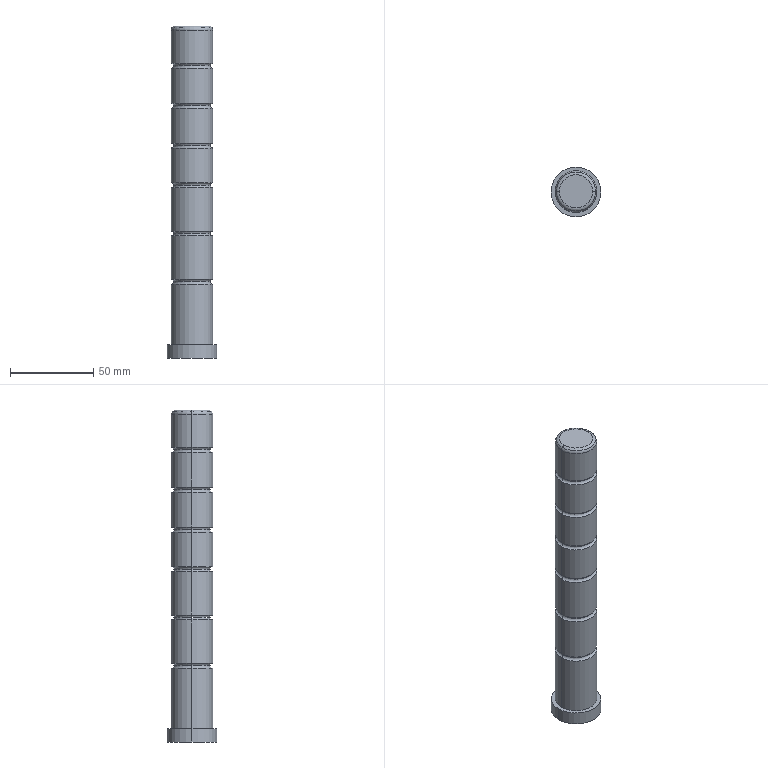Part | Creo | 1 solid | 54 faces | box 30 x 30 x 200 mm | volume 94808 mm3 | torus 28 | cylinder 20 | plane 4 | cone 2 | commonest cylinder face diameters 25 x14 10.2 x2 12 x2 30 x2
STEP:
#1=CARTESIAN_POINT('',(147.5,-266.,-182.));
#2=VERTEX_POINT('',#1);
#3=CARTESIAN_POINT('',(172.5,-266.,-182.));
#4=VERTEX_POINT('',#3);
#5=CARTESIAN_POINT('',(160.,-266.,-182.));
#6=DIRECTION('',(0.,0.,-1.));
#7=DIRECTION('',(-1.,0.,0.));
#8=AXIS2_PLACEMENT_3D('',#5,#6,#7);
#9=CIRCLE('',#8,12.5);
#10=EDGE_CURVE('',#2,#4,#9,.T.);
#11=ORIENTED_EDGE('',*,*,#10,.T.);
#12=CARTESIAN_POINT('',(172.5,-266.,-161.));
#13=VERTEX_POINT('',#12);
#14=CARTESIAN_POINT('',(172.5,-266.,-161.));
#15=DIRECTION('',(0.,0.,-1.));
#16=VECTOR('',#15,21.);
#17=LINE('',#14,#16);
#18=EDGE_CURVE('',#13,#4,#17,.T.);
#19=ORIENTED_EDGE('',*,*,#18,.F.);
#20=CARTESIAN_POINT('',(147.5,-266.,-161.));
#21=VERTEX_POINT('',#20);
#22=CARTESIAN_POINT('',(160.,-266.,-161.));
#23=DIRECTION('',(0.,0.,1.));
#24=DIRECTION('',(1.,0.,0.));
#25=AXIS2_PLACEMENT_3D('',#22,#23,#24);
#26=CIRCLE('',#25,12.5);
#27=EDGE_CURVE('',#13,#21,#26,.T.);
#28=ORIENTED_EDGE('',*,*,#27,.T.);
#29=CARTESIAN_POINT('',(147.5,-266.,-161.));
#30=DIRECTION('',(0.,0.,-1.));
#31=VECTOR('',#30,21.);
#32=LINE('',#29,#31);
#33=EDGE_CURVE('',#21,#2,#32,.T.);
#34=ORIENTED_EDGE('',*,*,#33,.T.);
#35=EDGE_LOOP('',(#11,#19,#28,#34));
#36=FACE_OUTER_BOUND('',#35,.F.);
#37=CARTESIAN_POINT('',(160.,-266.,-135.5));
#38=DIRECTION('',(0.,0.,-1.));
#39=DIRECTION('',(-1.,0.,0.));
#40=AXIS2_PLACEMENT_3D('',#37,#38,#39);
#41=CYLINDRICAL_SURFACE('',#40,12.5);
#42=ADVANCED_FACE('',(#36),#41,.T.);
#43=ORIENTED_EDGE('',*,*,#10,.F.);
#44=CARTESIAN_POINT('',(149.,-266.,-183.5));
#45=VERTEX_POINT('',#44);
#46=CARTESIAN_POINT('',(147.5,-266.,-183.5));
#47=DIRECTION('',(0.,1.,0.));
#48=DIRECTION('',(0.,0.,1.));
#49=AXIS2_PLACEMENT_3D('',#46,#47,#48);
#50=CIRCLE('',#49,1.5);
#51=EDGE_CURVE('',#2,#45,#50,.T.);
#52=ORIENTED_EDGE('',*,*,#51,.T.);
#53=CARTESIAN_POINT('',(171.,-266.,-183.5));
#54=VERTEX_POINT('',#53);
#55=CARTESIAN_POINT('',(160.,-266.,-183.5));
#56=DIRECTION('',(0.,0.,1.));
#57=DIRECTION('',(1.,0.,0.));
#58=AXIS2_PLACEMENT_3D('',#55,#56,#57);
#59=CIRCLE('',#58,11.);
#60=EDGE_CURVE('',#54,#45,#59,.T.);
#61=ORIENTED_EDGE('',*,*,#60,.F.);
#62=CARTESIAN_POINT('',(172.5,-266.,-183.5));
#63=DIRECTION('',(0.,-1.,0.));
#64=DIRECTION('',(0.,0.,1.));
#65=AXIS2_PLACEMENT_3D('',#62,#63,#64);
#66=CIRCLE('',#65,1.5);
#67=EDGE_CURVE('',#4,#54,#66,.T.);
#68=ORIENTED_EDGE('',*,*,#67,.F.);
#69=EDGE_LOOP('',(#43,#52,#61,#68));
#70=FACE_OUTER_BOUND('',#69,.F.);
#71=CARTESIAN_POINT('',(160.,-266.,-183.5));
#72=DIRECTION('',(0.,0.,1.));
#73=DIRECTION('',(1.,0.,0.));
#74=AXIS2_PLACEMENT_3D('',#71,#72,#73);
#75=TOROIDAL_SURFACE('',#74,12.5,1.5);
#76=ADVANCED_FACE('',(#70),#75,.F.);
#77=CARTESIAN_POINT('',(160.,-266.,-182.));
#78=DIRECTION('',(0.,0.,-1.));
#79=DIRECTION('',(1.,0.,0.));
#80=AXIS2_PLACEMENT_3D('',#77,#78,#79);
#81=CIRCLE('',#80,12.5);
#82=EDGE_CURVE('',#4,#2,#81,.T.);
#83=ORIENTED_EDGE('',*,*,#82,.F.);
#84=ORIENTED_EDGE('',*,*,#67,.T.);
#85=CARTESIAN_POINT('',(160.,-266.,-183.5));
#86=DIRECTION('',(0.,0.,1.));
#87=DIRECTION('',(-1.,0.,0.));
#88=AXIS2_PLACEMENT_3D('',#85,#86,#87);
#89=CIRCLE('',#88,11.);
#90=EDGE_CURVE('',#45,#54,#89,.T.);
#91=ORIENTED_EDGE('',*,*,#90,.F.);
#92=ORIENTED_EDGE('',*,*,#51,.F.);
#93=EDGE_LOOP('',(#83,#84,#91,#92));
#94=FACE_OUTER_BOUND('',#93,.F.);
#95=CARTESIAN_POINT('',(160.,-266.,-183.5));
#96=DIRECTION('',(0.,0.,1.));
#97=DIRECTION('',(1.,0.,0.));
#98=AXIS2_PLACEMENT_3D('',#95,#96,#97);
#99=TOROIDAL_SURFACE('',#98,12.5,1.5);
#100=ADVANCED_FACE('',(#94),#99,.F.);
#101=ORIENTED_EDGE('',*,*,#82,.T.);
#102=ORIENTED_EDGE('',*,*,#33,.F.);
#103=CARTESIAN_POINT('',(160.,-266.,-161.));
#104=DIRECTION('',(0.,0.,1.));
#105=DIRECTION('',(-1.,0.,0.));
#106=AXIS2_PLACEMENT_3D('',#103,#104,#105);
#107=CIRCLE('',#106,12.5);
#108=EDGE_CURVE('',#21,#13,#107,.T.);
#109=ORIENTED_EDGE('',*,*,#108,.T.);
#110=ORIENTED_EDGE('',*,*,#18,.T.);
#111=EDGE_LOOP('',(#101,#102,#109,#110));
#112=FACE_OUTER_BOUND('',#111,.F.);
#113=CARTESIAN_POINT('',(160.,-266.,-135.5));
#114=DIRECTION('',(0.,0.,-1.));
#115=DIRECTION('',(-1.,0.,0.));
#116=AXIS2_PLACEMENT_3D('',#113,#114,#115);
#117=CYLINDRICAL_SURFACE('',#116,12.5);
#118=ADVANCED_FACE('',(#112),#117,.T.);
#119=ORIENTED_EDGE('',*,*,#108,.F.);
#120=CARTESIAN_POINT('',(149.,-266.,-159.5));
#121=VERTEX_POINT('',#120);
#122=CARTESIAN_POINT('',(147.5,-266.,-159.5));
#123=DIRECTION('',(0.,1.,0.));
#124=DIRECTION('',(1.,0.,0.));
#125=AXIS2_PLACEMENT_3D('',#122,#123,#124);
#126=CIRCLE('',#125,1.5);
#127=EDGE_CURVE('',#121,#21,#126,.T.);
#128=ORIENTED_EDGE('',*,*,#127,.F.);
#129=CARTESIAN_POINT('',(171.,-266.,-159.5));
#130=VERTEX_POINT('',#129);
#131=CARTESIAN_POINT('',(160.,-266.,-159.5));
#132=DIRECTION('',(0.,0.,1.));
#133=DIRECTION('',(-1.,0.,0.));
#134=AXIS2_PLACEMENT_3D('',#131,#132,#133);
#135=CIRCLE('',#134,11.);
#136=EDGE_CURVE('',#121,#130,#135,.T.);
#137=ORIENTED_EDGE('',*,*,#136,.T.);
#138=CARTESIAN_POINT('',(172.5,-266.,-159.5));
#139=DIRECTION('',(0.,-1.,0.));
#140=DIRECTION('',(-1.,0.,0.));
#141=AXIS2_PLACEMENT_3D('',#138,#139,#140);
#142=CIRCLE('',#141,1.5);
#143=EDGE_CURVE('',#130,#13,#142,.T.);
#144=ORIENTED_EDGE('',*,*,#143,.T.);
#145=EDGE_LOOP('',(#119,#128,#137,#144));
#146=FACE_OUTER_BOUND('',#145,.F.);
#147=CARTESIAN_POINT('',(160.,-266.,-159.5));
#148=DIRECTION('',(0.,0.,1.));
#149=DIRECTION('',(1.,0.,0.));
#150=AXIS2_PLACEMENT_3D('',#147,#148,#149);
#151=TOROIDAL_SURFACE('',#150,12.5,1.5);
#152=ADVANCED_FACE('',(#146),#151,.F.);
#153=ORIENTED_EDGE('',*,*,#27,.F.);
#154=ORIENTED_EDGE('',*,*,#143,.F.);
#155=CARTESIAN_POINT('',(160.,-266.,-159.5));
#156=DIRECTION('',(0.,0.,1.));
#157=DIRECTION('',(1.,0.,0.));
#158=AXIS2_PLACEMENT_3D('',#155,#156,#157);
#159=CIRCLE('',#158,11.);
#160=EDGE_CURVE('',#130,#121,#159,.T.);
#161=ORIENTED_EDGE('',*,*,#160,.T.);
#162=ORIENTED_EDGE('',*,*,#127,.T.);
#163=EDGE_LOOP('',(#153,#154,#161,#162));
#164=FACE_OUTER_BOUND('',#163,.F.);
#165=CARTESIAN_POINT('',(160.,-266.,-159.5));
#166=DIRECTION('',(0.,0.,1.));
#167=DIRECTION('',(1.,0.,0.));
#168=AXIS2_PLACEMENT_3D('',#165,#166,#167);
#169=TOROIDAL_SURFACE('',#168,12.5,1.5);
#170=ADVANCED_FACE('',(#164),#169,.F.);
#171=CARTESIAN_POINT('',(147.5,-266.,-158.));
#172=VERTEX_POINT('',#171);
#173=CARTESIAN_POINT('',(172.5,-266.,-158.));
#174=VERTEX_POINT('',#173);
#175=CARTESIAN_POINT('',(160.,-266.,-158.));
#176=DIRECTION('',(0.,0.,-1.));
#177=DIRECTION('',(-1.,0.,0.));
#178=AXIS2_PLACEMENT_3D('',#175,#176,#177);
#179=CIRCLE('',#178,12.5);
#180=EDGE_CURVE('',#172,#174,#179,.T.);
#181=ORIENTED_EDGE('',*,*,#180,.F.);
#182=CARTESIAN_POINT('',(147.5,-266.,-159.5));
#183=DIRECTION('',(0.,1.,0.));
#184=DIRECTION('',(0.,0.,1.));
#185=AXIS2_PLACEMENT_3D('',#182,#183,#184);
#186=CIRCLE('',#185,1.5);
#187=EDGE_CURVE('',#172,#121,#186,.T.);
#188=ORIENTED_EDGE('',*,*,#187,.T.);
#189=ORIENTED_EDGE('',*,*,#160,.F.);
#190=CARTESIAN_POINT('',(172.5,-266.,-159.5));
#191=DIRECTION('',(0.,-1.,0.));
#192=DIRECTION('',(0.,0.,1.));
#193=AXIS2_PLACEMENT_3D('',#190,#191,#192);
#194=CIRCLE('',#193,1.5);
#195=EDGE_CURVE('',#174,#130,#194,.T.);
#196=ORIENTED_EDGE('',*,*,#195,.F.);
#197=EDGE_LOOP('',(#181,#188,#189,#196));
#198=FACE_OUTER_BOUND('',#197,.F.);
#199=CARTESIAN_POINT('',(160.,-266.,-159.5));
#200=DIRECTION('',(0.,0.,1.));
#201=DIRECTION('',(1.,0.,0.));
#202=AXIS2_PLACEMENT_3D('',#199,#200,#201);
#203=TOROIDAL_SURFACE('',#202,12.5,1.5);
#204=ADVANCED_FACE('',(#198),#203,.F.);
#205=CARTESIAN_POINT('',(172.5,-266.,-138.));
#206=VERTEX_POINT('',#205);
#207=CARTESIAN_POINT('',(147.5,-266.,-138.));
#208=VERTEX_POINT('',#207);
#209=CARTESIAN_POINT('',(160.,-266.,-138.));
#210=DIRECTION('',(0.,0.,1.));
#211=DIRECTION('',(1.,0.,0.));
#212=AXIS2_PLACEMENT_3D('',#209,#210,#211);
#213=CIRCLE('',#212,12.5);
#214=EDGE_CURVE('',#206,#208,#213,.T.);
#215=ORIENTED_EDGE('',*,*,#214,.T.);
#216=CARTESIAN_POINT('',(147.5,-266.,-138.));
#217=DIRECTION('',(0.,0.,-1.));
#218=VECTOR('',#217,20.);
#219=LINE('',#216,#218);
#220=EDGE_CURVE('',#208,#172,#219,.T.);
#221=ORIENTED_EDGE('',*,*,#220,.T.);
#222=ORIENTED_EDGE('',*,*,#180,.T.);
#223=CARTESIAN_POINT('',(172.5,-266.,-138.));
#224=DIRECTION('',(0.,0.,-1.));
#225=VECTOR('',#224,20.);
#226=LINE('',#223,#225);
#227=EDGE_CURVE('',#206,#174,#226,.T.);
#228=ORIENTED_EDGE('',*,*,#227,.F.);
#229=EDGE_LOOP('',(#215,#221,#222,#228));
#230=FACE_OUTER_BOUND('',#229,.F.);
#231=CARTESIAN_POINT('',(160.,-266.,-135.5));
#232=DIRECTION('',(0.,0.,-1.));
#233=DIRECTION('',(-1.,0.,0.));
#234=AXIS2_PLACEMENT_3D('',#231,#232,#233);
#235=CYLINDRICAL_SURFACE('',#234,12.5);
#236=ADVANCED_FACE('',(#230),#235,.T.);
#237=ORIENTED_EDGE('',*,*,#214,.F.);
#238=CARTESIAN_POINT('',(171.768,-266.,-136.232));
#239=VERTEX_POINT('',#238);
#240=CARTESIAN_POINT('',(170.,-266.,-138.));
#241=DIRECTION('',(0.,-1.,0.));
#242=DIRECTION('',(1.,0.,0.));
#243=AXIS2_PLACEMENT_3D('',#240,#241,#242);
#244=CIRCLE('',#243,2.5);
#245=EDGE_CURVE('',#206,#239,#244,.T.);
#246=ORIENTED_EDGE('',*,*,#245,.T.);
#247=CARTESIAN_POINT('',(148.232,-266.,-136.232));
#248=VERTEX_POINT('',#247);
#249=CARTESIAN_POINT('',(160.,-266.,-136.232));
#250=DIRECTION('',(0.,0.,1.));
#251=DIRECTION('',(1.,0.,0.));
#252=AXIS2_PLACEMENT_3D('',#249,#250,#251);
#253=CIRCLE('',#252,11.768);
#254=EDGE_CURVE('',#239,#248,#253,.T.);
#255=ORIENTED_EDGE('',*,*,#254,.T.);
#256=CARTESIAN_POINT('',(150.,-266.,-138.));
#257=DIRECTION('',(0.,1.,0.));
#258=DIRECTION('',(-1.,0.,0.));
#259=AXIS2_PLACEMENT_3D('',#256,#257,#258);
#260=CIRCLE('',#259,2.5);
#261=EDGE_CURVE('',#208,#248,#260,.T.);
#262=ORIENTED_EDGE('',*,*,#261,.F.);
#263=EDGE_LOOP('',(#237,#246,#255,#262));
#264=FACE_OUTER_BOUND('',#263,.F.);
#265=CARTESIAN_POINT('',(160.,-266.,-138.));
#266=DIRECTION('',(0.,0.,1.));
#267=DIRECTION('',(1.,0.,0.));
#268=AXIS2_PLACEMENT_3D('',#265,#266,#267);
#269=TOROIDAL_SURFACE('',#268,10.,2.5);
#270=ADVANCED_FACE('',(#264),#269,.T.);
#271=CARTESIAN_POINT('',(160.,-266.,-138.));
#272=DIRECTION('',(0.,0.,1.));
#273=DIRECTION('',(-1.,0.,0.));
#274=AXIS2_PLACEMENT_3D('',#271,#272,#273);
#275=CIRCLE('',#274,12.5);
#276=EDGE_CURVE('',#208,#206,#275,.T.);
#277=ORIENTED_EDGE('',*,*,#276,.F.);
#278=ORIENTED_EDGE('',*,*,#261,.T.);
#279=CARTESIAN_POINT('',(160.,-266.,-136.232));
#280=DIRECTION('',(0.,0.,1.));
#281=DIRECTION('',(-1.,0.,0.));
#282=AXIS2_PLACEMENT_3D('',#279,#280,#281);
#283=CIRCLE('',#282,11.768);
#284=EDGE_CURVE('',#248,#239,#283,.T.);
#285=ORIENTED_EDGE('',*,*,#284,.T.);
#286=ORIENTED_EDGE('',*,*,#245,.F.);
#287=EDGE_LOOP('',(#277,#278,#285,#286));
#288=FACE_OUTER_BOUND('',#287,.F.);
#289=CARTESIAN_POINT('',(160.,-266.,-138.));
#290=DIRECTION('',(0.,0.,1.));
#291=DIRECTION('',(1.,0.,0.));
#292=AXIS2_PLACEMENT_3D('',#289,#290,#291);
#293=TOROIDAL_SURFACE('',#292,10.,2.5);
#294=ADVANCED_FACE('',(#288),#293,.T.);
#295=ORIENTED_EDGE('',*,*,#276,.T.);
#296=ORIENTED_EDGE('',*,*,#227,.T.);
#297=CARTESIAN_POINT('',(160.,-266.,-158.));
#298=DIRECTION('',(0.,0.,-1.));
#299=DIRECTION('',(1.,0.,0.));
#300=AXIS2_PLACEMENT_3D('',#297,#298,#299);
#301=CIRCLE('',#300,12.5);
#302=EDGE_CURVE('',#174,#172,#301,.T.);
#303=ORIENTED_EDGE('',*,*,#302,.T.);
#304=ORIENTED_EDGE('',*,*,#220,.F.);
#305=EDGE_LOOP('',(#295,#296,#303,#304));
#306=FACE_OUTER_BOUND('',#305,.F.);
#307=CARTESIAN_POINT('',(160.,-266.,-135.5));
#308=DIRECTION('',(0.,0.,-1.));
#309=DIRECTION('',(-1.,0.,0.));
#310=AXIS2_PLACEMENT_3D('',#307,#308,#309);
#311=CYLINDRICAL_SURFACE('',#310,12.5);
#312=ADVANCED_FACE('',(#306),#311,.T.);
#313=ORIENTED_EDGE('',*,*,#302,.F.);
#314=ORIENTED_EDGE('',*,*,#195,.T.);
#315=ORIENTED_EDGE('',*,*,#136,.F.);
#316=ORIENTED_EDGE('',*,*,#187,.F.);
#317=EDGE_LOOP('',(#313,#314,#315,#316));
#318=FACE_OUTER_BOUND('',#317,.F.);
#319=CARTESIAN_POINT('',(160.,-266.,-159.5));
#320=DIRECTION('',(0.,0.,1.));
#321=DIRECTION('',(1.,0.,0.));
#322=AXIS2_PLACEMENT_3D('',#319,#320,#321);
#323=TOROIDAL_SURFACE('',#322,12.5,1.5);
#324=ADVANCED_FACE('',(#318),#323,.F.);
#325=CARTESIAN_POINT('',(150.,-266.,-135.5));
#326=VERTEX_POINT('',#325);
#327=CARTESIAN_POINT('',(170.,-266.,-135.5));
#328=VERTEX_POINT('',#327);
#329=CARTESIAN_POINT('',(160.,-266.,-135.5));
#330=DIRECTION('',(0.,0.,1.));
#331=DIRECTION('',(-1.,0.,0.));
#332=AXIS2_PLACEMENT_3D('',#329,#330,#331);
#333=CIRCLE('',#332,10.);
#334=EDGE_CURVE('',#326,#328,#333,.T.);
#335=ORIENTED_EDGE('',*,*,#334,.T.);
#336=CARTESIAN_POINT('',(170.,-266.,-138.));
#337=DIRECTION('',(0.,-1.,0.));
#338=DIRECTION('',(0.7071,0.,0.7071));
#339=AXIS2_PLACEMENT_3D('',#336,#337,#338);
#340=CIRCLE('',#339,2.5);
#341=EDGE_CURVE('',#239,#328,#340,.T.);
#342=ORIENTED_EDGE('',*,*,#341,.F.);
#343=ORIENTED_EDGE('',*,*,#284,.F.);
#344=CARTESIAN_POINT('',(150.,-266.,-138.));
#345=DIRECTION('',(0.,1.,0.));
#346=DIRECTION('',(-0.7071,0.,0.7071));
#347=AXIS2_PLACEMENT_3D('',#344,#345,#346);
#348=CIRCLE('',#347,2.5);
#349=EDGE_CURVE('',#248,#326,#348,.T.);
#350=ORIENTED_EDGE('',*,*,#349,.T.);
#351=EDGE_LOOP('',(#335,#342,#343,#350));
#352=FACE_OUTER_BOUND('',#351,.F.);
#353=CARTESIAN_POINT('',(160.,-266.,-138.));
#354=DIRECTION('',(0.,0.,1.));
#355=DIRECTION('',(1.,0.,0.));
#356=AXIS2_PLACEMENT_3D('',#353,#354,#355);
#357=TOROIDAL_SURFACE('',#356,10.,2.5);
#358=ADVANCED_FACE('',(#352),#357,.T.);
#359=CARTESIAN_POINT('',(160.,-266.,-135.5));
#360=DIRECTION('',(0.,0.,1.));
#361=DIRECTION('',(1.,0.,0.));
#362=AXIS2_PLACEMENT_3D('',#359,#360,#361);
#363=CIRCLE('',#362,10.);
#364=EDGE_CURVE('',#328,#326,#363,.T.);
#365=ORIENTED_EDGE('',*,*,#364,.F.);
#366=ORIENTED_EDGE('',*,*,#334,.F.);
#367=EDGE_LOOP('',(#365,#366));
#368=FACE_OUTER_BOUND('',#367,.F.);
#369=CARTESIAN_POINT('',(160.,-266.,-135.5));
#370=DIRECTION('',(0.,0.,1.));
#371=DIRECTION('',(1.,0.,0.));
#372=AXIS2_PLACEMENT_3D('',#369,#370,#371);
#373=PLANE('',#372);
#374=ADVANCED_FACE('',(#368),#373,.T.);
#375=ORIENTED_EDGE('',*,*,#364,.T.);
#376=ORIENTED_EDGE('',*,*,#349,.F.);
#377=ORIENTED_EDGE('',*,*,#254,.F.);
#378=ORIENTED_EDGE('',*,*,#341,.T.);
#379=EDGE_LOOP('',(#375,#376,#377,#378));
#380=FACE_OUTER_BOUND('',#379,.F.);
#381=CARTESIAN_POINT('',(160.,-266.,-138.));
#382=DIRECTION('',(0.,0.,1.));
#383=DIRECTION('',(1.,0.,0.));
#384=AXIS2_PLACEMENT_3D('',#381,#382,#383);
#385=TOROIDAL_SURFACE('',#384,10.,2.5);
#386=ADVANCED_FACE('',(#380),#385,.T.);
#387=CARTESIAN_POINT('',(147.5,-266.,-185.));
#388=VERTEX_POINT('',#387);
#389=CARTESIAN_POINT('',(172.5,-266.,-185.));
#390=VERTEX_POINT('',#389);
#391=CARTESIAN_POINT('',(160.,-266.,-185.));
#392=DIRECTION('',(0.,0.,1.));
#393=DIRECTION('',(-1.,0.,0.));
#394=AXIS2_PLACEMENT_3D('',#391,#392,#393);
#395=CIRCLE('',#394,12.5);
#396=EDGE_CURVE('',#388,#390,#395,.T.);
#397=ORIENTED_EDGE('',*,*,#396,.F.);
#398=CARTESIAN_POINT('',(147.5,-266.,-183.5));
#399=DIRECTION('',(0.,1.,0.));
#400=DIRECTION('',(1.,0.,0.));
#401=AXIS2_PLACEMENT_3D('',#398,#399,#400);
#402=CIRCLE('',#401,1.5);
#403=EDGE_CURVE('',#45,#388,#402,.T.);
#404=ORIENTED_EDGE('',*,*,#403,.F.);
#405=ORIENTED_EDGE('',*,*,#90,.T.);
#406=CARTESIAN_POINT('',(172.5,-266.,-183.5));
#407=DIRECTION('',(0.,-1.,0.));
#408=DIRECTION('',(-1.,0.,0.));
#409=AXIS2_PLACEMENT_3D('',#406,#407,#408);
#410=CIRCLE('',#409,1.5);
#411=EDGE_CURVE('',#54,#390,#410,.T.);
#412=ORIENTED_EDGE('',*,*,#411,.T.);
#413=EDGE_LOOP('',(#397,#404,#405,#412));
#414=FACE_OUTER_BOUND('',#413,.F.);
#415=CARTESIAN_POINT('',(160.,-266.,-183.5));
#416=DIRECTION('',(0.,0.,1.));
#417=DIRECTION('',(1.,0.,0.));
#418=AXIS2_PLACEMENT_3D('',#415,#416,#417);
#419=TOROIDAL_SURFACE('',#418,12.5,1.5);
#420=ADVANCED_FACE('',(#414),#419,.F.);
#421=CARTESIAN_POINT('',(172.5,-266.,-206.));
#422=VERTEX_POINT('',#421);
#423=CARTESIAN_POINT('',(147.5,-266.,-206.));
#424=VERTEX_POINT('',#423);
#425=CARTESIAN_POINT('',(160.,-266.,-206.));
#426=DIRECTION('',(0.,0.,-1.));
#427=DIRECTION('',(1.,0.,0.));
#428=AXIS2_PLACEMENT_3D('',#425,#426,#427);
#429=CIRCLE('',#428,12.5);
#430=EDGE_CURVE('',#422,#424,#429,.T.);
#431=ORIENTED_EDGE('',*,*,#430,.T.);
#432=CARTESIAN_POINT('',(147.5,-266.,-185.));
#433=DIRECTION('',(0.,0.,-1.));
#434=VECTOR('',#433,21.);
#435=LINE('',#432,#434);
#436=EDGE_CURVE('',#388,#424,#435,.T.);
#437=ORIENTED_EDGE('',*,*,#436,.F.);
#438=ORIENTED_EDGE('',*,*,#396,.T.);
#439=CARTESIAN_POINT('',(172.5,-266.,-185.));
#440=DIRECTION('',(0.,0.,-1.));
#441=VECTOR('',#440,21.);
#442=LINE('',#439,#441);
#443=EDGE_CURVE('',#390,#422,#442,.T.);
#444=ORIENTED_EDGE('',*,*,#443,.T.);
#445=EDGE_LOOP('',(#431,#437,#438,#444));
#446=FACE_OUTER_BOUND('',#445,.F.);
#447=CARTESIAN_POINT('',(160.,-266.,-135.5));
#448=DIRECTION('',(0.,0.,-1.));
#449=DIRECTION('',(-1.,0.,0.));
#450=AXIS2_PLACEMENT_3D('',#447,#448,#449);
#451=CYLINDRICAL_SURFACE('',#450,12.5);
#452=ADVANCED_FACE('',(#446),#451,.T.);
#453=ORIENTED_EDGE('',*,*,#430,.F.);
#454=CARTESIAN_POINT('',(171.,-266.,-207.5));
#455=VERTEX_POINT('',#454);
#456=CARTESIAN_POINT('',(172.5,-266.,-207.5));
#457=DIRECTION('',(0.,-1.,0.));
#458=DIRECTION('',(0.,0.,1.));
#459=AXIS2_PLACEMENT_3D('',#456,#457,#458);
#460=CIRCLE('',#459,1.5);
#461=EDGE_CURVE('',#422,#455,#460,.T.);
#462=ORIENTED_EDGE('',*,*,#461,.T.);
#463=CARTESIAN_POINT('',(149.,-266.,-207.5));
#464=VERTEX_POINT('',#463);
#465=CARTESIAN_POINT('',(160.,-266.,-207.5));
#466=DIRECTION('',(0.,0.,1.));
#467=DIRECTION('',(-1.,0.,0.));
#468=AXIS2_PLACEMENT_3D('',#465,#466,#467);
#469=CIRCLE('',#468,11.);
#470=EDGE_CURVE('',#464,#455,#469,.T.);
#471=ORIENTED_EDGE('',*,*,#470,.F.);
#472=CARTESIAN_POINT('',(147.5,-266.,-207.5));
#473=DIRECTION('',(0.,1.,0.));
#474=DIRECTION('',(0.,0.,1.));
#475=AXIS2_PLACEMENT_3D('',#472,#473,#474);
#476=CIRCLE('',#475,1.5);
#477=EDGE_CURVE('',#424,#464,#476,.T.);
#478=ORIENTED_EDGE('',*,*,#477,.F.);
#479=EDGE_LOOP('',(#453,#462,#471,#478));
#480=FACE_OUTER_BOUND('',#479,.F.);
#481=CARTESIAN_POINT('',(160.,-266.,-207.5));
#482=DIRECTION('',(0.,0.,1.));
#483=DIRECTION('',(1.,0.,0.));
#484=AXIS2_PLACEMENT_3D('',#481,#482,#483);
#485=TOROIDAL_SURFACE('',#484,12.5,1.5);
#486=ADVANCED_FACE('',(#480),#485,.F.);
#487=CARTESIAN_POINT('',(160.,-266.,-206.));
#488=DIRECTION('',(0.,0.,-1.));
#489=DIRECTION('',(-1.,0.,0.));
#490=AXIS2_PLACEMENT_3D('',#487,#488,#489);
#491=CIRCLE('',#490,12.5);
#492=EDGE_CURVE('',#424,#422,#491,.T.);
#493=ORIENTED_EDGE('',*,*,#492,.F.);
#494=ORIENTED_EDGE('',*,*,#477,.T.);
#495=CARTESIAN_POINT('',(160.,-266.,-207.5));
#496=DIRECTION('',(0.,0.,1.));
#497=DIRECTION('',(1.,0.,0.));
#498=AXIS2_PLACEMENT_3D('',#495,#496,#497);
#499=CIRCLE('',#498,11.);
#500=EDGE_CURVE('',#455,#464,#499,.T.);
#501=ORIENTED_EDGE('',*,*,#500,.F.);
#502=ORIENTED_EDGE('',*,*,#461,.F.);
#503=EDGE_LOOP('',(#493,#494,#501,#502));
#504=FACE_OUTER_BOUND('',#503,.F.);
#505=CARTESIAN_POINT('',(160.,-266.,-207.5));
#506=DIRECTION('',(0.,0.,1.));
#507=DIRECTION('',(1.,0.,0.));
#508=AXIS2_PLACEMENT_3D('',#505,#506,#507);
#509=TOROIDAL_SURFACE('',#508,12.5,1.5);
#510=ADVANCED_FACE('',(#504),#509,.F.);
#511=ORIENTED_EDGE('',*,*,#492,.T.);
#512=ORIENTED_EDGE('',*,*,#443,.F.);
#513=CARTESIAN_POINT('',(160.,-266.,-185.));
#514=DIRECTION('',(0.,0.,1.));
#515=DIRECTION('',(1.,0.,0.));
#516=AXIS2_PLACEMENT_3D('',#513,#514,#515);
#517=CIRCLE('',#516,12.5);
#518=EDGE_CURVE('',#390,#388,#517,.T.);
#519=ORIENTED_EDGE('',*,*,#518,.T.);
#520=ORIENTED_EDGE('',*,*,#436,.T.);
#521=EDGE_LOOP('',(#511,#512,#519,#520));
#522=FACE_OUTER_BOUND('',#521,.F.);
#523=CARTESIAN_POINT('',(160.,-266.,-135.5));
#524=DIRECTION('',(0.,0.,-1.));
#525=DIRECTION('',(-1.,0.,0.));
#526=AXIS2_PLACEMENT_3D('',#523,#524,#525);
#527=CYLINDRICAL_SURFACE('',#526,12.5);
#528=ADVANCED_FACE('',(#522),#527,.T.);
#529=ORIENTED_EDGE('',*,*,#518,.F.);
#530=ORIENTED_EDGE('',*,*,#411,.F.);
#531=ORIENTED_EDGE('',*,*,#60,.T.);
#532=ORIENTED_EDGE('',*,*,#403,.T.);
#533=EDGE_LOOP('',(#529,#530,#531,#532));
#534=FACE_OUTER_BOUND('',#533,.F.);
#535=CARTESIAN_POINT('',(160.,-266.,-183.5));
#536=DIRECTION('',(0.,0.,1.));
#537=DIRECTION('',(1.,0.,0.));
#538=AXIS2_PLACEMENT_3D('',#535,#536,#537);
#539=TOROIDAL_SURFACE('',#538,12.5,1.5);
#540=ADVANCED_FACE('',(#534),#539,.F.);
#541=CARTESIAN_POINT('',(172.5,-266.,-209.));
#542=VERTEX_POINT('',#541);
#543=CARTESIAN_POINT('',(147.5,-266.,-209.));
#544=VERTEX_POINT('',#543);
#545=CARTESIAN_POINT('',(160.,-266.,-209.));
#546=DIRECTION('',(0.,0.,1.));
#547=DIRECTION('',(1.,0.,0.));
#548=AXIS2_PLACEMENT_3D('',#545,#546,#547);
#549=CIRCLE('',#548,12.5);
#550=EDGE_CURVE('',#542,#544,#549,.T.);
#551=ORIENTED_EDGE('',*,*,#550,.F.);
#552=CARTESIAN_POINT('',(172.5,-266.,-207.5));
#553=DIRECTION('',(0.,-1.,0.));
#554=DIRECTION('',(-1.,0.,0.));
#555=AXIS2_PLACEMENT_3D('',#552,#553,#554);
#556=CIRCLE('',#555,1.5);
#557=EDGE_CURVE('',#455,#542,#556,.T.);
#558=ORIENTED_EDGE('',*,*,#557,.F.);
#559=ORIENTED_EDGE('',*,*,#500,.T.);
#560=CARTESIAN_POINT('',(147.5,-266.,-207.5));
#561=DIRECTION('',(0.,1.,0.));
#562=DIRECTION('',(1.,0.,0.));
#563=AXIS2_PLACEMENT_3D('',#560,#561,#562);
#564=CIRCLE('',#563,1.5);
#565=EDGE_CURVE('',#464,#544,#564,.T.);
#566=ORIENTED_EDGE('',*,*,#565,.T.);
#567=EDGE_LOOP('',(#551,#558,#559,#566));
#568=FACE_OUTER_BOUND('',#567,.F.);
#569=CARTESIAN_POINT('',(160.,-266.,-207.5));
#570=DIRECTION('',(0.,0.,1.));
#571=DIRECTION('',(1.,0.,0.));
#572=AXIS2_PLACEMENT_3D('',#569,#570,#571);
#573=TOROIDAL_SURFACE('',#572,12.5,1.5);
#574=ADVANCED_FACE('',(#568),#573,.F.);
#575=CARTESIAN_POINT('',(147.5,-266.,-230.));
#576=VERTEX_POINT('',#575);
#577=CARTESIAN_POINT('',(172.5,-266.,-230.));
#578=VERTEX_POINT('',#577);
#579=CARTESIAN_POINT('',(160.,-266.,-230.));
#580=DIRECTION('',(0.,0.,-1.));
#581=DIRECTION('',(-1.,0.,0.));
#582=AXIS2_PLACEMENT_3D('',#579,#580,#581);
#583=CIRCLE('',#582,12.5);
#584=EDGE_CURVE('',#576,#578,#583,.T.);
#585=ORIENTED_EDGE('',*,*,#584,.T.);
#586=CARTESIAN_POINT('',(172.5,-266.,-209.));
#587=DIRECTION('',(0.,0.,-1.));
#588=VECTOR('',#587,21.);
#589=LINE('',#586,#588);
#590=EDGE_CURVE('',#542,#578,#589,.T.);
#591=ORIENTED_EDGE('',*,*,#590,.F.);
#592=ORIENTED_EDGE('',*,*,#550,.T.);
#593=CARTESIAN_POINT('',(147.5,-266.,-209.));
#594=DIRECTION('',(0.,0.,-1.));
#595=VECTOR('',#594,21.);
#596=LINE('',#593,#595);
#597=EDGE_CURVE('',#544,#576,#596,.T.);
#598=ORIENTED_EDGE('',*,*,#597,.T.);
#599=EDGE_LOOP('',(#585,#591,#592,#598));
#600=FACE_OUTER_BOUND('',#599,.F.);
#601=CARTESIAN_POINT('',(160.,-266.,-135.5));
#602=DIRECTION('',(0.,0.,-1.));
#603=DIRECTION('',(-1.,0.,0.));
#604=AXIS2_PLACEMENT_3D('',#601,#602,#603);
#605=CYLINDRICAL_SURFACE('',#604,12.5);
#606=ADVANCED_FACE('',(#600),#605,.T.);
#607=ORIENTED_EDGE('',*,*,#584,.F.);
#608=CARTESIAN_POINT('',(149.,-266.,-231.5));
#609=VERTEX_POINT('',#608);
#610=CARTESIAN_POINT('',(147.5,-266.,-231.5));
#611=DIRECTION('',(0.,1.,0.));
#612=DIRECTION('',(0.,0.,1.));
#613=AXIS2_PLACEMENT_3D('',#610,#611,#612);
#614=CIRCLE('',#613,1.5);
#615=EDGE_CURVE('',#576,#609,#614,.T.);
#616=ORIENTED_EDGE('',*,*,#615,.T.);
#617=CARTESIAN_POINT('',(171.,-266.,-231.5));
#618=VERTEX_POINT('',#617);
#619=CARTESIAN_POINT('',(160.,-266.,-231.5));
#620=DIRECTION('',(0.,0.,1.));
#621=DIRECTION('',(1.,0.,0.));
#622=AXIS2_PLACEMENT_3D('',#619,#620,#621);
#623=CIRCLE('',#622,11.);
#624=EDGE_CURVE('',#618,#609,#623,.T.);
#625=ORIENTED_EDGE('',*,*,#624,.F.);
#626=CARTESIAN_POINT('',(172.5,-266.,-231.5));
#627=DIRECTION('',(0.,-1.,0.));
#628=DIRECTION('',(0.,0.,1.));
#629=AXIS2_PLACEMENT_3D('',#626,#627,#628);
#630=CIRCLE('',#629,1.5);
#631=EDGE_CURVE('',#578,#618,#630,.T.);
#632=ORIENTED_EDGE('',*,*,#631,.F.);
#633=EDGE_LOOP('',(#607,#616,#625,#632));
#634=FACE_OUTER_BOUND('',#633,.F.);
#635=CARTESIAN_POINT('',(160.,-266.,-231.5));
#636=DIRECTION('',(0.,0.,1.));
#637=DIRECTION('',(1.,0.,0.));
#638=AXIS2_PLACEMENT_3D('',#635,#636,#637);
#639=TOROIDAL_SURFACE('',#638,12.5,1.5);
#640=ADVANCED_FACE('',(#634),#639,.F.);
#641=CARTESIAN_POINT('',(160.,-266.,-230.));
#642=DIRECTION('',(0.,0.,-1.));
#643=DIRECTION('',(1.,0.,0.));
#644=AXIS2_PLACEMENT_3D('',#641,#642,#643);
#645=CIRCLE('',#644,12.5);
#646=EDGE_CURVE('',#578,#576,#645,.T.);
#647=ORIENTED_EDGE('',*,*,#646,.F.);
#648=ORIENTED_EDGE('',*,*,#631,.T.);
#649=CARTESIAN_POINT('',(160.,-266.,-231.5));
#650=DIRECTION('',(0.,0.,1.));
#651=DIRECTION('',(-1.,0.,0.));
#652=AXIS2_PLACEMENT_3D('',#649,#650,#651);
#653=CIRCLE('',#652,11.);
#654=EDGE_CURVE('',#609,#618,#653,.T.);
#655=ORIENTED_EDGE('',*,*,#654,.F.);
#656=ORIENTED_EDGE('',*,*,#615,.F.);
#657=EDGE_LOOP('',(#647,#648,#655,#656));
#658=FACE_OUTER_BOUND('',#657,.F.);
#659=CARTESIAN_POINT('',(160.,-266.,-231.5));
#660=DIRECTION('',(0.,0.,1.));
#661=DIRECTION('',(1.,0.,0.));
#662=AXIS2_PLACEMENT_3D('',#659,#660,#661);
#663=TOROIDAL_SURFACE('',#662,12.5,1.5);
#664=ADVANCED_FACE('',(#658),#663,.F.);
#665=ORIENTED_EDGE('',*,*,#646,.T.);
#666=ORIENTED_EDGE('',*,*,#597,.F.);
#667=CARTESIAN_POINT('',(160.,-266.,-209.));
#668=DIRECTION('',(0.,0.,1.));
#669=DIRECTION('',(-1.,0.,0.));
#670=AXIS2_PLACEMENT_3D('',#667,#668,#669);
#671=CIRCLE('',#670,12.5);
#672=EDGE_CURVE('',#544,#542,#671,.T.);
#673=ORIENTED_EDGE('',*,*,#672,.T.);
#674=ORIENTED_EDGE('',*,*,#590,.T.);
#675=EDGE_LOOP('',(#665,#666,#673,#674));
#676=FACE_OUTER_BOUND('',#675,.F.);
#677=CARTESIAN_POINT('',(160.,-266.,-135.5));
#678=DIRECTION('',(0.,0.,-1.));
#679=DIRECTION('',(-1.,0.,0.));
#680=AXIS2_PLACEMENT_3D('',#677,#678,#679);
#681=CYLINDRICAL_SURFACE('',#680,12.5);
#682=ADVANCED_FACE('',(#676),#681,.T.);
#683=ORIENTED_EDGE('',*,*,#672,.F.);
#684=ORIENTED_EDGE('',*,*,#565,.F.);
#685=ORIENTED_EDGE('',*,*,#470,.T.);
#686=ORIENTED_EDGE('',*,*,#557,.T.);
#687=EDGE_LOOP('',(#683,#684,#685,#686));
#688=FACE_OUTER_BOUND('',#687,.F.);
#689=CARTESIAN_POINT('',(160.,-266.,-207.5));
#690=DIRECTION('',(0.,0.,1.));
#691=DIRECTION('',(1.,0.,0.));
#692=AXIS2_PLACEMENT_3D('',#689,#690,#691);
#693=TOROIDAL_SURFACE('',#692,12.5,1.5);
#694=ADVANCED_FACE('',(#688),#693,.F.);
#695=CARTESIAN_POINT('',(147.5,-266.,-233.));
#696=VERTEX_POINT('',#695);
#697=CARTESIAN_POINT('',(172.5,-266.,-233.));
#698=VERTEX_POINT('',#697);
#699=CARTESIAN_POINT('',(160.,-266.,-233.));
#700=DIRECTION('',(0.,0.,1.));
#701=DIRECTION('',(-1.,0.,0.));
#702=AXIS2_PLACEMENT_3D('',#699,#700,#701);
#703=CIRCLE('',#702,12.5);
#704=EDGE_CURVE('',#696,#698,#703,.T.);
#705=ORIENTED_EDGE('',*,*,#704,.F.);
#706=CARTESIAN_POINT('',(147.5,-266.,-231.5));
#707=DIRECTION('',(0.,1.,0.));
#708=DIRECTION('',(1.,0.,0.));
#709=AXIS2_PLACEMENT_3D('',#706,#707,#708);
#710=CIRCLE('',#709,1.5);
#711=EDGE_CURVE('',#609,#696,#710,.T.);
#712=ORIENTED_EDGE('',*,*,#711,.F.);
#713=ORIENTED_EDGE('',*,*,#654,.T.);
#714=CARTESIAN_POINT('',(172.5,-266.,-231.5));
#715=DIRECTION('',(0.,-1.,0.));
#716=DIRECTION('',(-1.,0.,0.));
#717=AXIS2_PLACEMENT_3D('',#714,#715,#716);
#718=CIRCLE('',#717,1.5);
#719=EDGE_CURVE('',#618,#698,#718,.T.);
#720=ORIENTED_EDGE('',*,*,#719,.T.);
#721=EDGE_LOOP('',(#705,#712,#713,#720));
#722=FACE_OUTER_BOUND('',#721,.F.);
#723=CARTESIAN_POINT('',(160.,-266.,-231.5));
#724=DIRECTION('',(0.,0.,1.));
#725=DIRECTION('',(1.,0.,0.));
#726=AXIS2_PLACEMENT_3D('',#723,#724,#725);
#727=TOROIDAL_SURFACE('',#726,12.5,1.5);
#728=ADVANCED_FACE('',(#722),#727,.F.);
#729=CARTESIAN_POINT('',(172.5,-266.,-259.));
#730=VERTEX_POINT('',#729);
#731=CARTESIAN_POINT('',(147.5,-266.,-259.));
#732=VERTEX_POINT('',#731);
#733=CARTESIAN_POINT('',(160.,-266.,-259.));
#734=DIRECTION('',(0.,0.,-1.));
#735=DIRECTION('',(1.,0.,0.));
#736=AXIS2_PLACEMENT_3D('',#733,#734,#735);
#737=CIRCLE('',#736,12.5);
#738=EDGE_CURVE('',#730,#732,#737,.T.);
#739=ORIENTED_EDGE('',*,*,#738,.T.);
#740=CARTESIAN_POINT('',(147.5,-266.,-233.));
#741=DIRECTION('',(0.,0.,-1.));
#742=VECTOR('',#741,26.);
#743=LINE('',#740,#742);
#744=EDGE_CURVE('',#696,#732,#743,.T.);
#745=ORIENTED_EDGE('',*,*,#744,.F.);
#746=ORIENTED_EDGE('',*,*,#704,.T.);
#747=CARTESIAN_POINT('',(172.5,-266.,-233.));
#748=DIRECTION('',(0.,0.,-1.));
#749=VECTOR('',#748,26.);
#750=LINE('',#747,#749);
#751=EDGE_CURVE('',#698,#730,#750,.T.);
#752=ORIENTED_EDGE('',*,*,#751,.T.);
#753=EDGE_LOOP('',(#739,#745,#746,#752));
#754=FACE_OUTER_BOUND('',#753,.F.);
#755=CARTESIAN_POINT('',(160.,-266.,-135.5));
#756=DIRECTION('',(0.,0.,-1.));
#757=DIRECTION('',(-1.,0.,0.));
#758=AXIS2_PLACEMENT_3D('',#755,#756,#757);
#759=CYLINDRICAL_SURFACE('',#758,12.5);
#760=ADVANCED_FACE('',(#754),#759,.T.);
#761=ORIENTED_EDGE('',*,*,#738,.F.);
#762=CARTESIAN_POINT('',(171.,-266.,-260.5));
#763=VERTEX_POINT('',#762);
#764=CARTESIAN_POINT('',(172.5,-266.,-260.5));
#765=DIRECTION('',(0.,-1.,0.));
#766=DIRECTION('',(0.,0.,1.));
#767=AXIS2_PLACEMENT_3D('',#764,#765,#766);
#768=CIRCLE('',#767,1.5);
#769=EDGE_CURVE('',#730,#763,#768,.T.);
#770=ORIENTED_EDGE('',*,*,#769,.T.);
#771=CARTESIAN_POINT('',(149.,-266.,-260.5));
#772=VERTEX_POINT('',#771);
#773=CARTESIAN_POINT('',(160.,-266.,-260.5));
#774=DIRECTION('',(0.,0.,1.));
#775=DIRECTION('',(-1.,0.,0.));
#776=AXIS2_PLACEMENT_3D('',#773,#774,#775);
#777=CIRCLE('',#776,11.);
#778=EDGE_CURVE('',#772,#763,#777,.T.);
#779=ORIENTED_EDGE('',*,*,#778,.F.);
#780=CARTESIAN_POINT('',(147.5,-266.,-260.5));
#781=DIRECTION('',(0.,1.,0.));
#782=DIRECTION('',(0.,0.,1.));
#783=AXIS2_PLACEMENT_3D('',#780,#781,#782);
#784=CIRCLE('',#783,1.5);
#785=EDGE_CURVE('',#732,#772,#784,.T.);
#786=ORIENTED_EDGE('',*,*,#785,.F.);
#787=EDGE_LOOP('',(#761,#770,#779,#786));
#788=FACE_OUTER_BOUND('',#787,.F.);
#789=CARTESIAN_POINT('',(160.,-266.,-260.5));
#790=DIRECTION('',(0.,0.,1.));
#791=DIRECTION('',(1.,0.,0.));
#792=AXIS2_PLACEMENT_3D('',#789,#790,#791);
#793=TOROIDAL_SURFACE('',#792,12.5,1.5);
#794=ADVANCED_FACE('',(#788),#793,.F.);
#795=CARTESIAN_POINT('',(160.,-266.,-259.));
#796=DIRECTION('',(0.,0.,-1.));
#797=DIRECTION('',(-1.,0.,0.));
#798=AXIS2_PLACEMENT_3D('',#795,#796,#797);
#799=CIRCLE('',#798,12.5);
#800=EDGE_CURVE('',#732,#730,#799,.T.);
#801=ORIENTED_EDGE('',*,*,#800,.F.);
#802=ORIENTED_EDGE('',*,*,#785,.T.);
#803=CARTESIAN_POINT('',(160.,-266.,-260.5));
#804=DIRECTION('',(0.,0.,1.));
#805=DIRECTION('',(1.,0.,0.));
#806=AXIS2_PLACEMENT_3D('',#803,#804,#805);
#807=CIRCLE('',#806,11.);
#808=EDGE_CURVE('',#763,#772,#807,.T.);
#809=ORIENTED_EDGE('',*,*,#808,.F.);
#810=ORIENTED_EDGE('',*,*,#769,.F.);
#811=EDGE_LOOP('',(#801,#802,#809,#810));
#812=FACE_OUTER_BOUND('',#811,.F.);
#813=CARTESIAN_POINT('',(160.,-266.,-260.5));
#814=DIRECTION('',(0.,0.,1.));
#815=DIRECTION('',(1.,0.,0.));
#816=AXIS2_PLACEMENT_3D('',#813,#814,#815);
#817=TOROIDAL_SURFACE('',#816,12.5,1.5);
#818=ADVANCED_FACE('',(#812),#817,.F.);
#819=ORIENTED_EDGE('',*,*,#800,.T.);
#820=ORIENTED_EDGE('',*,*,#751,.F.);
#821=CARTESIAN_POINT('',(160.,-266.,-233.));
#822=DIRECTION('',(0.,0.,1.));
#823=DIRECTION('',(1.,0.,0.));
#824=AXIS2_PLACEMENT_3D('',#821,#822,#823);
#825=CIRCLE('',#824,12.5);
#826=EDGE_CURVE('',#698,#696,#825,.T.);
#827=ORIENTED_EDGE('',*,*,#826,.T.);
#828=ORIENTED_EDGE('',*,*,#744,.T.);
#829=EDGE_LOOP('',(#819,#820,#827,#828));
#830=FACE_OUTER_BOUND('',#829,.F.);
#831=CARTESIAN_POINT('',(160.,-266.,-135.5));
#832=DIRECTION('',(0.,0.,-1.));
#833=DIRECTION('',(-1.,0.,0.));
#834=AXIS2_PLACEMENT_3D('',#831,#832,#833);
#835=CYLINDRICAL_SURFACE('',#834,12.5);
#836=ADVANCED_FACE('',(#830),#835,.T.);
#837=ORIENTED_EDGE('',*,*,#826,.F.);
#838=ORIENTED_EDGE('',*,*,#719,.F.);
#839=ORIENTED_EDGE('',*,*,#624,.T.);
#840=ORIENTED_EDGE('',*,*,#711,.T.);
#841=EDGE_LOOP('',(#837,#838,#839,#840));
#842=FACE_OUTER_BOUND('',#841,.F.);
#843=CARTESIAN_POINT('',(160.,-266.,-231.5));
#844=DIRECTION('',(0.,0.,1.));
#845=DIRECTION('',(1.,0.,0.));
#846=AXIS2_PLACEMENT_3D('',#843,#844,#845);
#847=TOROIDAL_SURFACE('',#846,12.5,1.5);
#848=ADVANCED_FACE('',(#842),#847,.F.);
#849=CARTESIAN_POINT('',(172.5,-266.,-262.));
#850=VERTEX_POINT('',#849);
#851=CARTESIAN_POINT('',(147.5,-266.,-262.));
#852=VERTEX_POINT('',#851);
#853=CARTESIAN_POINT('',(160.,-266.,-262.));
#854=DIRECTION('',(0.,0.,1.));
#855=DIRECTION('',(1.,0.,0.));
#856=AXIS2_PLACEMENT_3D('',#853,#854,#855);
#857=CIRCLE('',#856,12.5);
#858=EDGE_CURVE('',#850,#852,#857,.T.);
#859=ORIENTED_EDGE('',*,*,#858,.F.);
#860=CARTESIAN_POINT('',(172.5,-266.,-260.5));
#861=DIRECTION('',(0.,-1.,0.));
#862=DIRECTION('',(-1.,0.,0.));
#863=AXIS2_PLACEMENT_3D('',#860,#861,#862);
#864=CIRCLE('',#863,1.5);
#865=EDGE_CURVE('',#763,#850,#864,.T.);
#866=ORIENTED_EDGE('',*,*,#865,.F.);
#867=ORIENTED_EDGE('',*,*,#808,.T.);
#868=CARTESIAN_POINT('',(147.5,-266.,-260.5));
#869=DIRECTION('',(0.,1.,0.));
#870=DIRECTION('',(1.,0.,0.));
#871=AXIS2_PLACEMENT_3D('',#868,#869,#870);
#872=CIRCLE('',#871,1.5);
#873=EDGE_CURVE('',#772,#852,#872,.T.);
#874=ORIENTED_EDGE('',*,*,#873,.T.);
#875=EDGE_LOOP('',(#859,#866,#867,#874));
#876=FACE_OUTER_BOUND('',#875,.F.);
#877=CARTESIAN_POINT('',(160.,-266.,-260.5));
#878=DIRECTION('',(0.,0.,1.));
#879=DIRECTION('',(1.,0.,0.));
#880=AXIS2_PLACEMENT_3D('',#877,#878,#879);
#881=TOROIDAL_SURFACE('',#880,12.5,1.5);
#882=ADVANCED_FACE('',(#876),#881,.F.);
#883=CARTESIAN_POINT('',(147.5,-266.,-288.));
#884=VERTEX_POINT('',#883);
#885=CARTESIAN_POINT('',(172.5,-266.,-288.));
#886=VERTEX_POINT('',#885);
#887=CARTESIAN_POINT('',(160.,-266.,-288.));
#888=DIRECTION('',(0.,0.,-1.));
#889=DIRECTION('',(-1.,0.,0.));
#890=AXIS2_PLACEMENT_3D('',#887,#888,#889);
#891=CIRCLE('',#890,12.5);
#892=EDGE_CURVE('',#884,#886,#891,.T.);
#893=ORIENTED_EDGE('',*,*,#892,.T.);
#894=CARTESIAN_POINT('',(172.5,-266.,-262.));
#895=DIRECTION('',(0.,0.,-1.));
#896=VECTOR('',#895,26.);
#897=LINE('',#894,#896);
#898=EDGE_CURVE('',#850,#886,#897,.T.);
#899=ORIENTED_EDGE('',*,*,#898,.F.);
#900=ORIENTED_EDGE('',*,*,#858,.T.);
#901=CARTESIAN_POINT('',(147.5,-266.,-262.));
#902=DIRECTION('',(0.,0.,-1.));
#903=VECTOR('',#902,26.);
#904=LINE('',#901,#903);
#905=EDGE_CURVE('',#852,#884,#904,.T.);
#906=ORIENTED_EDGE('',*,*,#905,.T.);
#907=EDGE_LOOP('',(#893,#899,#900,#906));
#908=FACE_OUTER_BOUND('',#907,.F.);
#909=CARTESIAN_POINT('',(160.,-266.,-145.5));
#910=DIRECTION('',(0.,0.,-1.));
#911=DIRECTION('',(-1.,0.,0.));
#912=AXIS2_PLACEMENT_3D('',#909,#910,#911);
#913=CYLINDRICAL_SURFACE('',#912,12.5);
#914=ADVANCED_FACE('',(#908),#913,.T.);
#915=ORIENTED_EDGE('',*,*,#892,.F.);
#916=CARTESIAN_POINT('',(149.,-266.,-289.5));
#917=VERTEX_POINT('',#916);
#918=CARTESIAN_POINT('',(147.5,-266.,-289.5));
#919=DIRECTION('',(0.,1.,0.));
#920=DIRECTION('',(0.,0.,1.));
#921=AXIS2_PLACEMENT_3D('',#918,#919,#920);
#922=CIRCLE('',#921,1.5);
#923=EDGE_CURVE('',#884,#917,#922,.T.);
#924=ORIENTED_EDGE('',*,*,#923,.T.);
#925=CARTESIAN_POINT('',(171.,-266.,-289.5));
#926=VERTEX_POINT('',#925);
#927=CARTESIAN_POINT('',(160.,-266.,-289.5));
#928=DIRECTION('',(0.,0.,1.));
#929=DIRECTION('',(1.,0.,0.));
#930=AXIS2_PLACEMENT_3D('',#927,#928,#929);
#931=CIRCLE('',#930,11.);
#932=EDGE_CURVE('',#926,#917,#931,.T.);
#933=ORIENTED_EDGE('',*,*,#932,.F.);
#934=CARTESIAN_POINT('',(172.5,-266.,-289.5));
#935=DIRECTION('',(0.,-1.,0.));
#936=DIRECTION('',(0.,0.,1.));
#937=AXIS2_PLACEMENT_3D('',#934,#935,#936);
#938=CIRCLE('',#937,1.5);
#939=EDGE_CURVE('',#886,#926,#938,.T.);
#940=ORIENTED_EDGE('',*,*,#939,.F.);
#941=EDGE_LOOP('',(#915,#924,#933,#940));
#942=FACE_OUTER_BOUND('',#941,.F.);
#943=CARTESIAN_POINT('',(160.,-266.,-289.5));
#944=DIRECTION('',(0.,0.,1.));
#945=DIRECTION('',(1.,0.,0.));
#946=AXIS2_PLACEMENT_3D('',#943,#944,#945);
#947=TOROIDAL_SURFACE('',#946,12.5,1.5);
#948=ADVANCED_FACE('',(#942),#947,.F.);
#949=CARTESIAN_POINT('',(160.,-266.,-288.));
#950=DIRECTION('',(0.,0.,-1.));
#951=DIRECTION('',(1.,0.,0.));
#952=AXIS2_PLACEMENT_3D('',#949,#950,#951);
#953=CIRCLE('',#952,12.5);
#954=EDGE_CURVE('',#886,#884,#953,.T.);
#955=ORIENTED_EDGE('',*,*,#954,.F.);
#956=ORIENTED_EDGE('',*,*,#939,.T.);
#957=CARTESIAN_POINT('',(160.,-266.,-289.5));
#958=DIRECTION('',(0.,0.,1.));
#959=DIRECTION('',(-1.,0.,0.));
#960=AXIS2_PLACEMENT_3D('',#957,#958,#959);
#961=CIRCLE('',#960,11.);
#962=EDGE_CURVE('',#917,#926,#961,.T.);
#963=ORIENTED_EDGE('',*,*,#962,.F.);
#964=ORIENTED_EDGE('',*,*,#923,.F.);
#965=EDGE_LOOP('',(#955,#956,#963,#964));
#966=FACE_OUTER_BOUND('',#965,.F.);
#967=CARTESIAN_POINT('',(160.,-266.,-289.5));
#968=DIRECTION('',(0.,0.,1.));
#969=DIRECTION('',(1.,0.,0.));
#970=AXIS2_PLACEMENT_3D('',#967,#968,#969);
#971=TOROIDAL_SURFACE('',#970,12.5,1.5);
#972=ADVANCED_FACE('',(#966),#971,.F.);
#973=ORIENTED_EDGE('',*,*,#954,.T.);
#974=ORIENTED_EDGE('',*,*,#905,.F.);
#975=CARTESIAN_POINT('',(160.,-266.,-262.));
#976=DIRECTION('',(0.,0.,1.));
#977=DIRECTION('',(-1.,0.,0.));
#978=AXIS2_PLACEMENT_3D('',#975,#976,#977);
#979=CIRCLE('',#978,12.5);
#980=EDGE_CURVE('',#852,#850,#979,.T.);
#981=ORIENTED_EDGE('',*,*,#980,.T.);
#982=ORIENTED_EDGE('',*,*,#898,.T.);
#983=EDGE_LOOP('',(#973,#974,#981,#982));
#984=FACE_OUTER_BOUND('',#983,.F.);
#985=CARTESIAN_POINT('',(160.,-266.,-145.5));
#986=DIRECTION('',(0.,0.,-1.));
#987=DIRECTION('',(-1.,0.,0.));
#988=AXIS2_PLACEMENT_3D('',#985,#986,#987);
#989=CYLINDRICAL_SURFACE('',#988,12.5);
#990=ADVANCED_FACE('',(#984),#989,.T.);
#991=ORIENTED_EDGE('',*,*,#980,.F.);
#992=ORIENTED_EDGE('',*,*,#873,.F.);
#993=ORIENTED_EDGE('',*,*,#778,.T.);
#994=ORIENTED_EDGE('',*,*,#865,.T.);
#995=EDGE_LOOP('',(#991,#992,#993,#994));
#996=FACE_OUTER_BOUND('',#995,.F.);
#997=CARTESIAN_POINT('',(160.,-266.,-260.5));
#998=DIRECTION('',(0.,0.,1.));
#999=DIRECTION('',(1.,0.,0.));
#1000=AXIS2_PLACEMENT_3D('',#997,#998,#999);
#1001=TOROIDAL_SURFACE('',#1000,12.5,1.5);
#1002=ADVANCED_FACE('',(#996),#1001,.F.);
#1003=CARTESIAN_POINT('',(147.5,-266.,-291.));
#1004=VERTEX_POINT('',#1003);
#1005=CARTESIAN_POINT('',(172.5,-266.,-291.));
#1006=VERTEX_POINT('',#1005);
#1007=CARTESIAN_POINT('',(160.,-266.,-291.));
#1008=DIRECTION('',(0.,0.,1.));
#1009=DIRECTION('',(-1.,0.,0.));
#1010=AXIS2_PLACEMENT_3D('',#1007,#1008,#1009);
#1011=CIRCLE('',#1010,12.5);
#1012=EDGE_CURVE('',#1004,#1006,#1011,.T.);
#1013=ORIENTED_EDGE('',*,*,#1012,.F.);
#1014=CARTESIAN_POINT('',(147.5,-266.,-289.5));
#1015=DIRECTION('',(0.,1.,0.));
#1016=DIRECTION('',(1.,0.,0.));
#1017=AXIS2_PLACEMENT_3D('',#1014,#1015,#1016);
#1018=CIRCLE('',#1017,1.5);
#1019=EDGE_CURVE('',#917,#1004,#1018,.T.);
#1020=ORIENTED_EDGE('',*,*,#1019,.F.);
#1021=ORIENTED_EDGE('',*,*,#962,.T.);
#1022=CARTESIAN_POINT('',(172.5,-266.,-289.5));
#1023=DIRECTION('',(0.,-1.,0.));
#1024=DIRECTION('',(-1.,0.,0.));
#1025=AXIS2_PLACEMENT_3D('',#1022,#1023,#1024);
#1026=CIRCLE('',#1025,1.5);
#1027=EDGE_CURVE('',#926,#1006,#1026,.T.);
#1028=ORIENTED_EDGE('',*,*,#1027,.T.);
#1029=EDGE_LOOP('',(#1013,#1020,#1021,#1028));
#1030=FACE_OUTER_BOUND('',#1029,.F.);
#1031=CARTESIAN_POINT('',(160.,-266.,-289.5));
#1032=DIRECTION('',(0.,0.,1.));
#1033=DIRECTION('',(1.,0.,0.));
#1034=AXIS2_PLACEMENT_3D('',#1031,#1032,#1033);
#1035=TOROIDAL_SURFACE('',#1034,12.5,1.5);
#1036=ADVANCED_FACE('',(#1030),#1035,.F.);
#1037=CARTESIAN_POINT('',(172.5,-266.,-327.5));
#1038=VERTEX_POINT('',#1037);
#1039=CARTESIAN_POINT('',(147.5,-266.,-327.5));
#1040=VERTEX_POINT('',#1039);
#1041=CARTESIAN_POINT('',(160.,-266.,-327.5));
#1042=DIRECTION('',(0.,0.,-1.));
#1043=DIRECTION('',(1.,0.,0.));
#1044=AXIS2_PLACEMENT_3D('',#1041,#1042,#1043);
#1045=CIRCLE('',#1044,12.5);
#1046=EDGE_CURVE('',#1038,#1040,#1045,.T.);
#1047=ORIENTED_EDGE('',*,*,#1046,.T.);
#1048=CARTESIAN_POINT('',(147.5,-266.,-291.));
#1049=DIRECTION('',(0.,0.,-1.));
#1050=VECTOR('',#1049,36.5);
#1051=LINE('',#1048,#1050);
#1052=EDGE_CURVE('',#1004,#1040,#1051,.T.);
#1053=ORIENTED_EDGE('',*,*,#1052,.F.);
#1054=ORIENTED_EDGE('',*,*,#1012,.T.);
#1055=CARTESIAN_POINT('',(172.5,-266.,-291.));
#1056=DIRECTION('',(0.,0.,-1.));
#1057=VECTOR('',#1056,36.5);
#1058=LINE('',#1055,#1057);
#1059=EDGE_CURVE('',#1006,#1038,#1058,.T.);
#1060=ORIENTED_EDGE('',*,*,#1059,.T.);
#1061=EDGE_LOOP('',(#1047,#1053,#1054,#1060));
#1062=FACE_OUTER_BOUND('',#1061,.F.);
#1063=CARTESIAN_POINT('',(160.,-266.,-145.5));
#1064=DIRECTION('',(0.,0.,-1.));
#1065=DIRECTION('',(-1.,0.,0.));
#1066=AXIS2_PLACEMENT_3D('',#1063,#1064,#1065);
#1067=CYLINDRICAL_SURFACE('',#1066,12.5);
#1068=ADVANCED_FACE('',(#1062),#1067,.T.);
#1069=CARTESIAN_POINT('',(145.,-266.,-327.5));
#1070=VERTEX_POINT('',#1069);
#1071=CARTESIAN_POINT('',(175.,-266.,-327.5));
#1072=VERTEX_POINT('',#1071);
#1073=CARTESIAN_POINT('',(160.,-266.,-327.5));
#1074=DIRECTION('',(0.,0.,1.));
#1075=DIRECTION('',(-1.,0.,0.));
#1076=AXIS2_PLACEMENT_3D('',#1073,#1074,#1075);
#1077=CIRCLE('',#1076,15.);
#1078=EDGE_CURVE('',#1070,#1072,#1077,.T.);
#1079=ORIENTED_EDGE('',*,*,#1078,.F.);
#1080=CARTESIAN_POINT('',(160.,-266.,-327.5));
#1081=DIRECTION('',(0.,0.,1.));
#1082=DIRECTION('',(1.,0.,0.));
#1083=AXIS2_PLACEMENT_3D('',#1080,#1081,#1082);
#1084=CIRCLE('',#1083,15.);
#1085=EDGE_CURVE('',#1072,#1070,#1084,.T.);
#1086=ORIENTED_EDGE('',*,*,#1085,.F.);
#1087=EDGE_LOOP('',(#1079,#1086));
#1088=FACE_OUTER_BOUND('',#1087,.F.);
#1089=ORIENTED_EDGE('',*,*,#1046,.F.);
#1090=CARTESIAN_POINT('',(160.,-266.,-327.5));
#1091=DIRECTION('',(0.,0.,-1.));
#1092=DIRECTION('',(-1.,0.,0.));
#1093=AXIS2_PLACEMENT_3D('',#1090,#1091,#1092);
#1094=CIRCLE('',#1093,12.5);
#1095=EDGE_CURVE('',#1040,#1038,#1094,.T.);
#1096=ORIENTED_EDGE('',*,*,#1095,.F.);
#1097=EDGE_LOOP('',(#1089,#1096));
#1098=FACE_BOUND('',#1097,.F.);
#1099=CARTESIAN_POINT('',(160.,-266.,-327.5));
#1100=DIRECTION('',(0.,0.,1.));
#1101=DIRECTION('',(1.,0.,0.));
#1102=AXIS2_PLACEMENT_3D('',#1099,#1100,#1101);
#1103=PLANE('',#1102);
#1104=ADVANCED_FACE('',(#1088,#1098),#1103,.T.);
#1105=ORIENTED_EDGE('',*,*,#1095,.T.);
#1106=ORIENTED_EDGE('',*,*,#1059,.F.);
#1107=CARTESIAN_POINT('',(160.,-266.,-291.));
#1108=DIRECTION('',(0.,0.,1.));
#1109=DIRECTION('',(1.,0.,0.));
#1110=AXIS2_PLACEMENT_3D('',#1107,#1108,#1109);
#1111=CIRCLE('',#1110,12.5);
#1112=EDGE_CURVE('',#1006,#1004,#1111,.T.);
#1113=ORIENTED_EDGE('',*,*,#1112,.T.);
#1114=ORIENTED_EDGE('',*,*,#1052,.T.);
#1115=EDGE_LOOP('',(#1105,#1106,#1113,#1114));
#1116=FACE_OUTER_BOUND('',#1115,.F.);
#1117=CARTESIAN_POINT('',(160.,-266.,-145.5));
#1118=DIRECTION('',(0.,0.,-1.));
#1119=DIRECTION('',(-1.,0.,0.));
#1120=AXIS2_PLACEMENT_3D('',#1117,#1118,#1119);
#1121=CYLINDRICAL_SURFACE('',#1120,12.5);
#1122=ADVANCED_FACE('',(#1116),#1121,.T.);
#1123=ORIENTED_EDGE('',*,*,#1112,.F.);
#1124=ORIENTED_EDGE('',*,*,#1027,.F.);
#1125=ORIENTED_EDGE('',*,*,#932,.T.);
#1126=ORIENTED_EDGE('',*,*,#1019,.T.);
#1127=EDGE_LOOP('',(#1123,#1124,#1125,#1126));
#1128=FACE_OUTER_BOUND('',#1127,.F.);
#1129=CARTESIAN_POINT('',(160.,-266.,-289.5));
#1130=DIRECTION('',(0.,0.,1.));
#1131=DIRECTION('',(1.,0.,0.));
#1132=AXIS2_PLACEMENT_3D('',#1129,#1130,#1131);
#1133=TOROIDAL_SURFACE('',#1132,12.5,1.5);
#1134=ADVANCED_FACE('',(#1128),#1133,.F.);
#1135=ORIENTED_EDGE('',*,*,#1078,.T.);
#1136=CARTESIAN_POINT('',(175.,-266.,-335.5));
#1137=VERTEX_POINT('',#1136);
#1138=CARTESIAN_POINT('',(175.,-266.,-335.5));
#1139=DIRECTION('',(0.,0.,1.));
#1140=VECTOR('',#1139,8.);
#1141=LINE('',#1138,#1140);
#1142=EDGE_CURVE('',#1137,#1072,#1141,.T.);
#1143=ORIENTED_EDGE('',*,*,#1142,.F.);
#1144=CARTESIAN_POINT('',(145.,-266.,-335.5));
#1145=VERTEX_POINT('',#1144);
#1146=CARTESIAN_POINT('',(160.,-266.,-335.5));
#1147=DIRECTION('',(0.,0.,-1.));
#1148=DIRECTION('',(1.,0.,0.));
#1149=AXIS2_PLACEMENT_3D('',#1146,#1147,#1148);
#1150=CIRCLE('',#1149,15.);
#1151=EDGE_CURVE('',#1137,#1145,#1150,.T.);
#1152=ORIENTED_EDGE('',*,*,#1151,.T.);
#1153=CARTESIAN_POINT('',(145.,-266.,-335.5));
#1154=DIRECTION('',(0.,0.,1.));
#1155=VECTOR('',#1154,8.);
#1156=LINE('',#1153,#1155);
#1157=EDGE_CURVE('',#1145,#1070,#1156,.T.);
#1158=ORIENTED_EDGE('',*,*,#1157,.T.);
#1159=EDGE_LOOP('',(#1135,#1143,#1152,#1158));
#1160=FACE_OUTER_BOUND('',#1159,.F.);
#1161=CARTESIAN_POINT('',(160.,-266.,-335.5));
#1162=DIRECTION('',(0.,0.,1.));
#1163=DIRECTION('',(1.,0.,0.));
#1164=AXIS2_PLACEMENT_3D('',#1161,#1162,#1163);
#1165=CYLINDRICAL_SURFACE('',#1164,15.);
#1166=ADVANCED_FACE('',(#1160),#1165,.T.);
#1167=ORIENTED_EDGE('',*,*,#1085,.T.);
#1168=ORIENTED_EDGE('',*,*,#1157,.F.);
#1169=CARTESIAN_POINT('',(160.,-266.,-335.5));
#1170=DIRECTION('',(0.,0.,-1.));
#1171=DIRECTION('',(-1.,0.,0.));
#1172=AXIS2_PLACEMENT_3D('',#1169,#1170,#1171);
#1173=CIRCLE('',#1172,15.);
#1174=EDGE_CURVE('',#1145,#1137,#1173,.T.);
#1175=ORIENTED_EDGE('',*,*,#1174,.T.);
#1176=ORIENTED_EDGE('',*,*,#1142,.T.);
#1177=EDGE_LOOP('',(#1167,#1168,#1175,#1176));
#1178=FACE_OUTER_BOUND('',#1177,.F.);
#1179=CARTESIAN_POINT('',(160.,-266.,-335.5));
#1180=DIRECTION('',(0.,0.,1.));
#1181=DIRECTION('',(1.,0.,0.));
#1182=AXIS2_PLACEMENT_3D('',#1179,#1180,#1181);
#1183=CYLINDRICAL_SURFACE('',#1182,15.);
#1184=ADVANCED_FACE('',(#1178),#1183,.T.);
#1185=ORIENTED_EDGE('',*,*,#1151,.F.);
#1186=ORIENTED_EDGE('',*,*,#1174,.F.);
#1187=EDGE_LOOP('',(#1185,#1186));
#1188=FACE_OUTER_BOUND('',#1187,.F.);
#1189=CARTESIAN_POINT('',(166.,-266.,-335.5));
#1190=VERTEX_POINT('',#1189);
#1191=CARTESIAN_POINT('',(154.,-266.,-335.5));
#1192=VERTEX_POINT('',#1191);
#1193=CARTESIAN_POINT('',(160.,-266.,-335.5));
#1194=DIRECTION('',(0.,0.,1.));
#1195=DIRECTION('',(1.,0.,0.));
#1196=AXIS2_PLACEMENT_3D('',#1193,#1194,#1195);
#1197=CIRCLE('',#1196,6.);
#1198=EDGE_CURVE('',#1190,#1192,#1197,.T.);
#1199=ORIENTED_EDGE('',*,*,#1198,.F.);
#1200=CARTESIAN_POINT('',(160.,-266.,-335.5));
#1201=DIRECTION('',(0.,0.,1.));
#1202=DIRECTION('',(-1.,0.,0.));
#1203=AXIS2_PLACEMENT_3D('',#1200,#1201,#1202);
#1204=CIRCLE('',#1203,6.);
#1205=EDGE_CURVE('',#1192,#1190,#1204,.T.);
#1206=ORIENTED_EDGE('',*,*,#1205,.F.);
#1207=EDGE_LOOP('',(#1199,#1206));
#1208=FACE_BOUND('',#1207,.F.);
#1209=CARTESIAN_POINT('',(160.,-266.,-335.5));
#1210=DIRECTION('',(0.,0.,-1.));
#1211=DIRECTION('',(-1.,0.,0.));
#1212=AXIS2_PLACEMENT_3D('',#1209,#1210,#1211);
#1213=PLANE('',#1212);
#1214=ADVANCED_FACE('',(#1188,#1208),#1213,.T.);
#1215=CARTESIAN_POINT('',(154.,-266.,-307.5));
#1216=VERTEX_POINT('',#1215);
#1217=CARTESIAN_POINT('',(166.,-266.,-307.5));
#1218=VERTEX_POINT('',#1217);
#1219=CARTESIAN_POINT('',(160.,-266.,-307.5));
#1220=DIRECTION('',(0.,0.,-1.));
#1221=DIRECTION('',(-1.,0.,0.));
#1222=AXIS2_PLACEMENT_3D('',#1219,#1220,#1221);
#1223=CIRCLE('',#1222,6.);
#1224=EDGE_CURVE('',#1216,#1218,#1223,.T.);
#1225=ORIENTED_EDGE('',*,*,#1224,.T.);
#1226=CARTESIAN_POINT('',(166.,-266.,-335.5));
#1227=DIRECTION('',(0.,0.,1.));
#1228=VECTOR('',#1227,28.);
#1229=LINE('',#1226,#1228);
#1230=EDGE_CURVE('',#1190,#1218,#1229,.T.);
#1231=ORIENTED_EDGE('',*,*,#1230,.F.);
#1232=ORIENTED_EDGE('',*,*,#1198,.T.);
#1233=CARTESIAN_POINT('',(154.,-266.,-335.5));
#1234=DIRECTION('',(0.,0.,1.));
#1235=VECTOR('',#1234,28.);
#1236=LINE('',#1233,#1235);
#1237=EDGE_CURVE('',#1192,#1216,#1236,.T.);
#1238=ORIENTED_EDGE('',*,*,#1237,.T.);
#1239=EDGE_LOOP('',(#1225,#1231,#1232,#1238));
#1240=FACE_OUTER_BOUND('',#1239,.F.);
#1241=CARTESIAN_POINT('',(160.,-266.,-335.5));
#1242=DIRECTION('',(0.,0.,1.));
#1243=DIRECTION('',(1.,0.,0.));
#1244=AXIS2_PLACEMENT_3D('',#1241,#1242,#1243);
#1245=CYLINDRICAL_SURFACE('',#1244,6.);
#1246=ADVANCED_FACE('',(#1240),#1245,.F.);
#1247=ORIENTED_EDGE('',*,*,#1224,.F.);
#1248=CARTESIAN_POINT('',(160.,-266.,-307.5));
#1249=DIRECTION('',(0.,0.,-1.));
#1250=DIRECTION('',(1.,0.,0.));
#1251=AXIS2_PLACEMENT_3D('',#1248,#1249,#1250);
#1252=CIRCLE('',#1251,6.);
#1253=EDGE_CURVE('',#1218,#1216,#1252,.T.);
#1254=ORIENTED_EDGE('',*,*,#1253,.F.);
#1255=EDGE_LOOP('',(#1247,#1254));
#1256=FACE_OUTER_BOUND('',#1255,.F.);
#1257=CARTESIAN_POINT('',(165.1,-266.,-307.5));
#1258=VERTEX_POINT('',#1257);
#1259=CARTESIAN_POINT('',(154.9,-266.,-307.5));
#1260=VERTEX_POINT('',#1259);
#1261=CARTESIAN_POINT('',(160.,-266.,-307.5));
#1262=DIRECTION('',(0.,0.,1.));
#1263=DIRECTION('',(1.,0.,0.));
#1264=AXIS2_PLACEMENT_3D('',#1261,#1262,#1263);
#1265=CIRCLE('',#1264,5.1);
#1266=EDGE_CURVE('',#1258,#1260,#1265,.T.);
#1267=ORIENTED_EDGE('',*,*,#1266,.F.);
#1268=CARTESIAN_POINT('',(160.,-266.,-307.5));
#1269=DIRECTION('',(0.,0.,1.));
#1270=DIRECTION('',(-1.,0.,0.));
#1271=AXIS2_PLACEMENT_3D('',#1268,#1269,#1270);
#1272=CIRCLE('',#1271,5.1);
#1273=EDGE_CURVE('',#1260,#1258,#1272,.T.);
#1274=ORIENTED_EDGE('',*,*,#1273,.F.);
#1275=EDGE_LOOP('',(#1267,#1274));
#1276=FACE_BOUND('',#1275,.F.);
#1277=CARTESIAN_POINT('',(160.,-266.,-307.5));
#1278=DIRECTION('',(0.,0.,1.));
#1279=DIRECTION('',(1.,0.,0.));
#1280=AXIS2_PLACEMENT_3D('',#1277,#1278,#1279);
#1281=PLANE('',#1280);
#1282=ADVANCED_FACE('',(#1256,#1276),#1281,.F.);
#1283=CARTESIAN_POINT('',(154.9,-266.,-305.5));
#1284=VERTEX_POINT('',#1283);
#1285=CARTESIAN_POINT('',(165.1,-266.,-305.5));
#1286=VERTEX_POINT('',#1285);
#1287=CARTESIAN_POINT('',(160.,-266.,-305.5));
#1288=DIRECTION('',(0.,0.,-1.));
#1289=DIRECTION('',(-1.,0.,0.));
#1290=AXIS2_PLACEMENT_3D('',#1287,#1288,#1289);
#1291=CIRCLE('',#1290,5.1);
#1292=EDGE_CURVE('',#1284,#1286,#1291,.T.);
#1293=ORIENTED_EDGE('',*,*,#1292,.T.);
#1294=CARTESIAN_POINT('',(165.1,-266.,-307.5));
#1295=DIRECTION('',(0.,0.,1.));
#1296=VECTOR('',#1295,2.);
#1297=LINE('',#1294,#1296);
#1298=EDGE_CURVE('',#1258,#1286,#1297,.T.);
#1299=ORIENTED_EDGE('',*,*,#1298,.F.);
#1300=ORIENTED_EDGE('',*,*,#1266,.T.);
#1301=CARTESIAN_POINT('',(154.9,-266.,-307.5));
#1302=DIRECTION('',(0.,0.,1.));
#1303=VECTOR('',#1302,2.);
#1304=LINE('',#1301,#1303);
#1305=EDGE_CURVE('',#1260,#1284,#1304,.T.);
#1306=ORIENTED_EDGE('',*,*,#1305,.T.);
#1307=EDGE_LOOP('',(#1293,#1299,#1300,#1306));
#1308=FACE_OUTER_BOUND('',#1307,.F.);
#1309=CARTESIAN_POINT('',(160.,-266.,-335.5));
#1310=DIRECTION('',(0.,0.,1.));
#1311=DIRECTION('',(1.,0.,0.));
#1312=AXIS2_PLACEMENT_3D('',#1309,#1310,#1311);
#1313=CYLINDRICAL_SURFACE('',#1312,5.1);
#1314=ADVANCED_FACE('',(#1308),#1313,.F.);
#1315=ORIENTED_EDGE('',*,*,#1292,.F.);
#1316=CARTESIAN_POINT('',(160.,-266.,-302.436));
#1317=VERTEX_POINT('',#1316);
#1318=CARTESIAN_POINT('',(160.,-266.,-302.436));
#1319=DIRECTION('',(-0.8572,0.,-0.515));
#1320=VECTOR('',#1319,5.95);
#1321=LINE('',#1318,#1320);
#1322=EDGE_CURVE('',#1317,#1284,#1321,.T.);
#1323=ORIENTED_EDGE('',*,*,#1322,.F.);
#1324=CARTESIAN_POINT('',(160.,-266.,-302.436));
#1325=DIRECTION('',(0.8572,0.,-0.515));
#1326=VECTOR('',#1325,5.95);
#1327=LINE('',#1324,#1326);
#1328=EDGE_CURVE('',#1317,#1286,#1327,.T.);
#1329=ORIENTED_EDGE('',*,*,#1328,.T.);
#1330=EDGE_LOOP('',(#1315,#1323,#1329));
#1331=FACE_OUTER_BOUND('',#1330,.F.);
#1332=CARTESIAN_POINT('',(160.,-266.,-304.031));
#1333=DIRECTION('',(0.,0.,-1.));
#1334=DIRECTION('',(-1.,0.,0.));
#1335=AXIS2_PLACEMENT_3D('',#1332,#1333,#1334);
#1336=CONICAL_SURFACE('',#1335,2.655,59.);
#1337=ADVANCED_FACE('',(#1331),#1336,.F.);
#1338=CARTESIAN_POINT('',(160.,-266.,-305.5));
#1339=DIRECTION('',(0.,0.,-1.));
#1340=DIRECTION('',(1.,0.,0.));
#1341=AXIS2_PLACEMENT_3D('',#1338,#1339,#1340);
#1342=CIRCLE('',#1341,5.1);
#1343=EDGE_CURVE('',#1286,#1284,#1342,.T.);
#1344=ORIENTED_EDGE('',*,*,#1343,.F.);
#1345=ORIENTED_EDGE('',*,*,#1328,.F.);
#1346=ORIENTED_EDGE('',*,*,#1322,.T.);
#1347=EDGE_LOOP('',(#1344,#1345,#1346));
#1348=FACE_OUTER_BOUND('',#1347,.F.);
#1349=CARTESIAN_POINT('',(160.,-266.,-304.031));
#1350=DIRECTION('',(0.,0.,-1.));
#1351=DIRECTION('',(-1.,0.,0.));
#1352=AXIS2_PLACEMENT_3D('',#1349,#1350,#1351);
#1353=CONICAL_SURFACE('',#1352,2.655,59.);
#1354=ADVANCED_FACE('',(#1348),#1353,.F.);
#1355=ORIENTED_EDGE('',*,*,#1343,.T.);
#1356=ORIENTED_EDGE('',*,*,#1305,.F.);
#1357=ORIENTED_EDGE('',*,*,#1273,.T.);
#1358=ORIENTED_EDGE('',*,*,#1298,.T.);
#1359=EDGE_LOOP('',(#1355,#1356,#1357,#1358));
#1360=FACE_OUTER_BOUND('',#1359,.F.);
#1361=CARTESIAN_POINT('',(160.,-266.,-335.5));
#1362=DIRECTION('',(0.,0.,1.));
#1363=DIRECTION('',(1.,0.,0.));
#1364=AXIS2_PLACEMENT_3D('',#1361,#1362,#1363);
#1365=CYLINDRICAL_SURFACE('',#1364,5.1);
#1366=ADVANCED_FACE('',(#1360),#1365,.F.);
#1367=ORIENTED_EDGE('',*,*,#1253,.T.);
#1368=ORIENTED_EDGE('',*,*,#1237,.F.);
#1369=ORIENTED_EDGE('',*,*,#1205,.T.);
#1370=ORIENTED_EDGE('',*,*,#1230,.T.);
#1371=EDGE_LOOP('',(#1367,#1368,#1369,#1370));
#1372=FACE_OUTER_BOUND('',#1371,.F.);
#1373=CARTESIAN_POINT('',(160.,-266.,-335.5));
#1374=DIRECTION('',(0.,0.,1.));
#1375=DIRECTION('',(1.,0.,0.));
#1376=AXIS2_PLACEMENT_3D('',#1373,#1374,#1375);
#1377=CYLINDRICAL_SURFACE('',#1376,6.);
#1378=ADVANCED_FACE('',(#1372),#1377,.F.);
#1379=CLOSED_SHELL('',(#42,#76,#100,#118,#152,#170,#204,#236,#270,#294,#312,#324,#358,#374,#386,#420,#452,#486,#510,#528,#540,#574,#606,#640,#664,#682,#694,#728,#760,#794,#818,#836,#848,#882,#914,#948,#972,#990,#1002,#1036,#1068,#1104,#1122,#1134,#1166,#1184,#1214,#1246,#1282,#1314,#1337,#1354,#1366,#1378));
#1380=MANIFOLD_SOLID_BREP('',#1379);
#1381=(LENGTH_UNIT()NAMED_UNIT(*)SI_UNIT(.MILLI.,.METRE.));
#1382=UNCERTAINTY_MEASURE_WITH_UNIT(LENGTH_MEASURE(0.02044),#1381,'','');
#1383=(NAMED_UNIT(*)PLANE_ANGLE_UNIT()SI_UNIT($,.RADIAN.));
#1384=PLANE_ANGLE_MEASURE_WITH_UNIT(PLANE_ANGLE_MEASURE(0.01745),#1383);
#1385=(CONVERSION_BASED_UNIT('DEGREE',#1384)NAMED_UNIT(*)PLANE_ANGLE_UNIT());
#1386=(NAMED_UNIT(*)SI_UNIT($,.STERADIAN.)SOLID_ANGLE_UNIT());
#1387=(GEOMETRIC_REPRESENTATION_CONTEXT(3)GLOBAL_UNCERTAINTY_ASSIGNED_CONTEXT((#1382))GLOBAL_UNIT_ASSIGNED_CONTEXT((#1381,#1385,#1386))REPRESENTATION_CONTEXT('',''));
#1388=ADVANCED_BREP_SHAPE_REPRESENTATION('',(#1380),#1387);